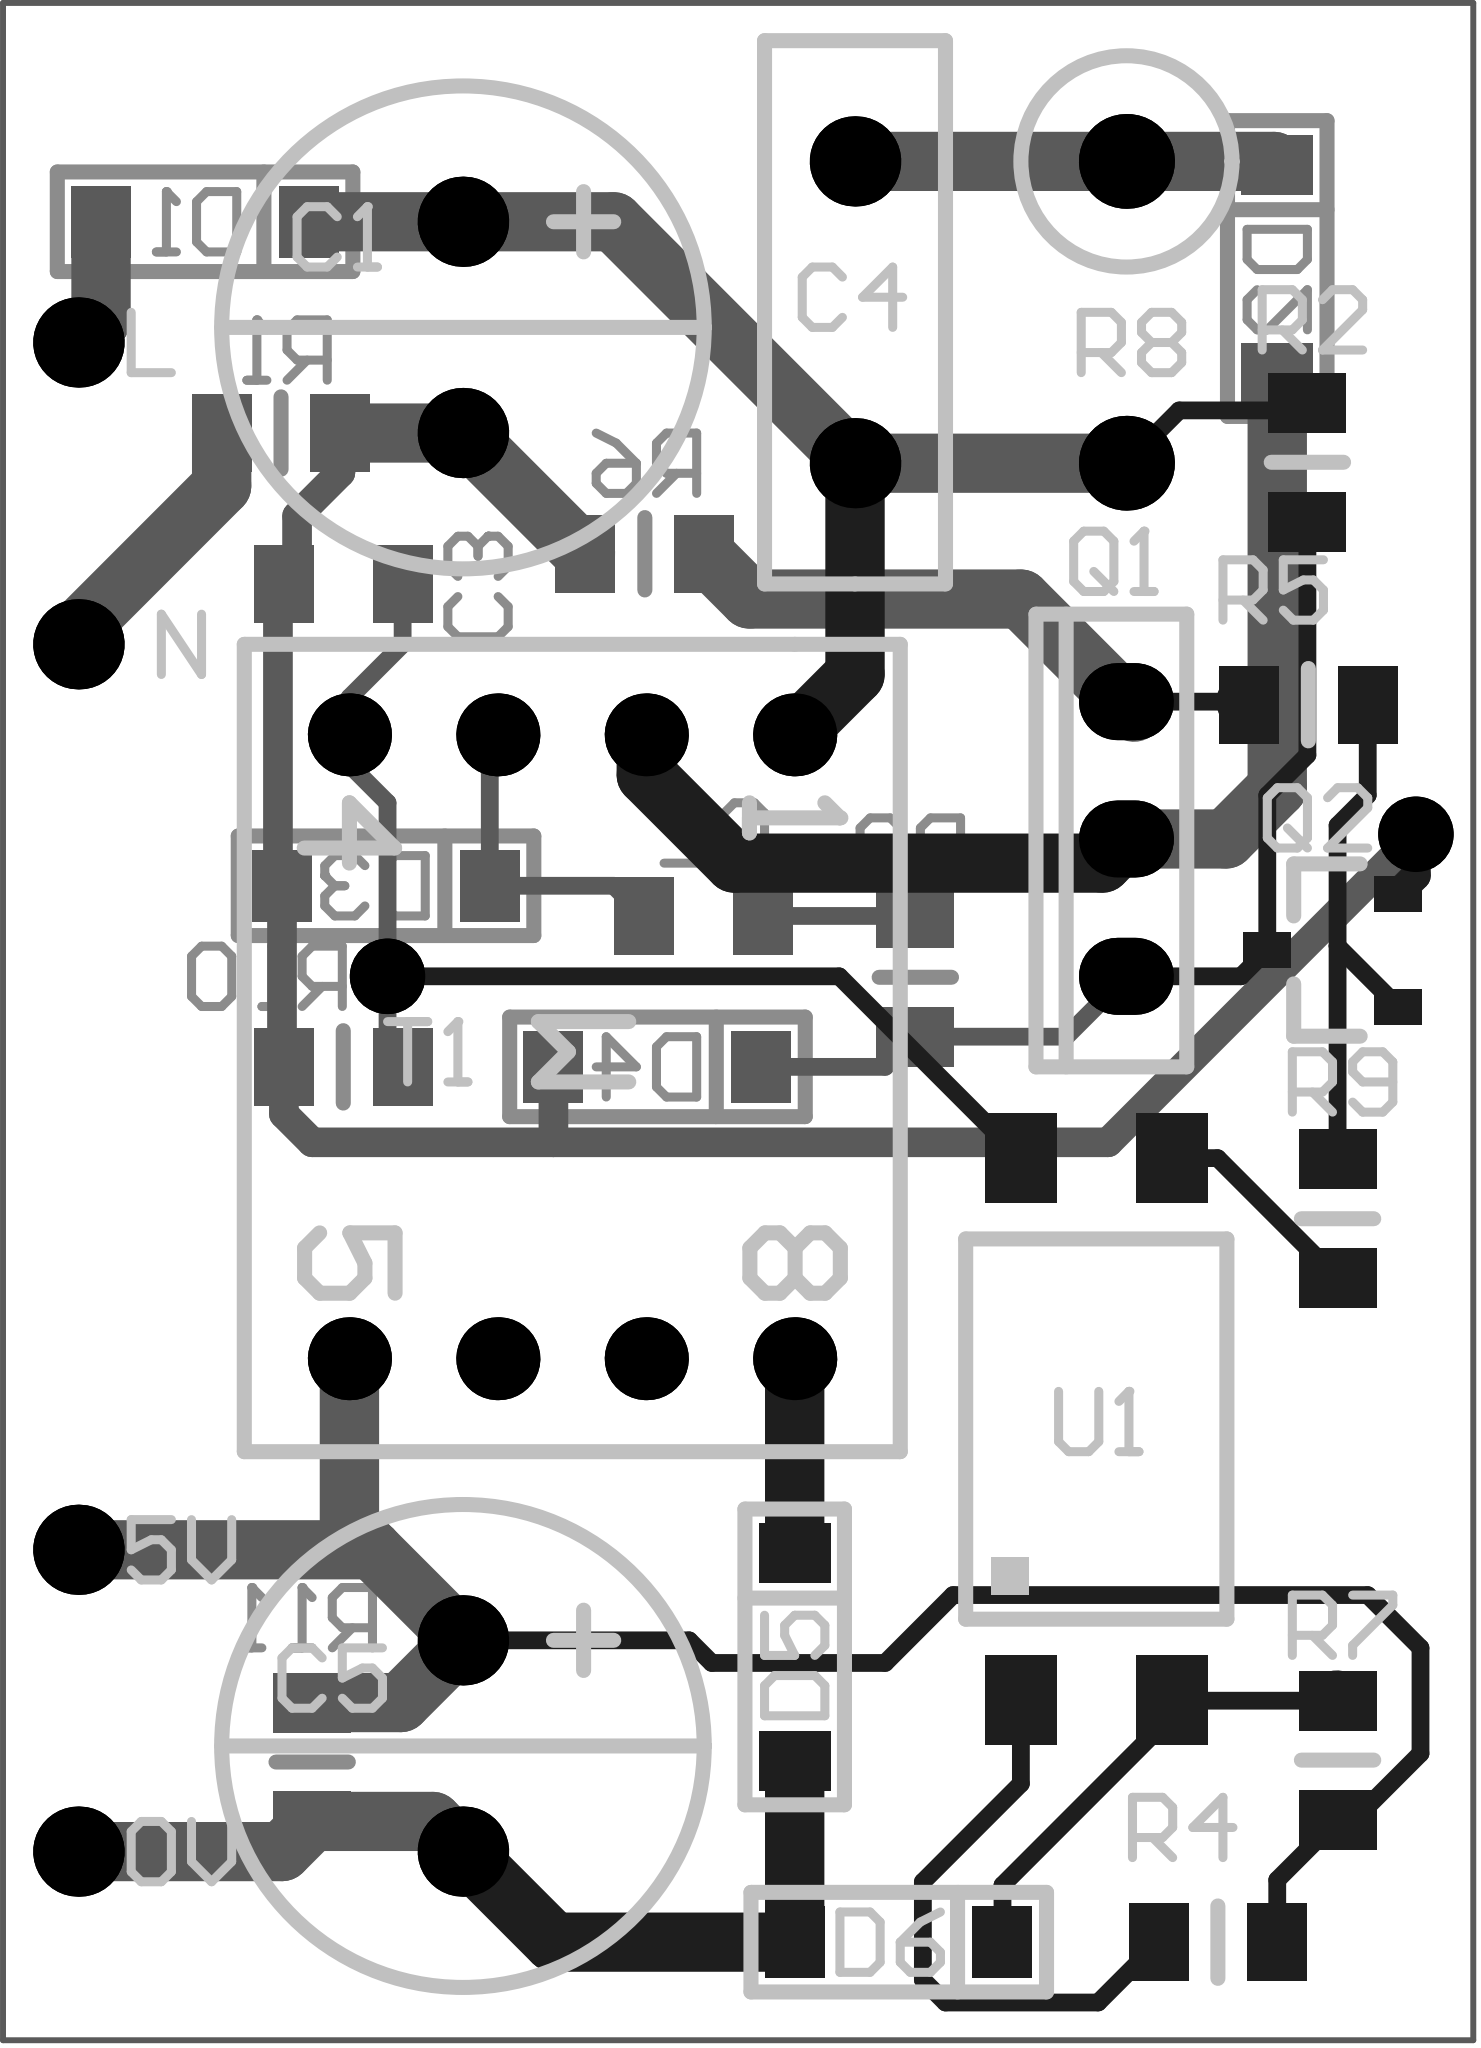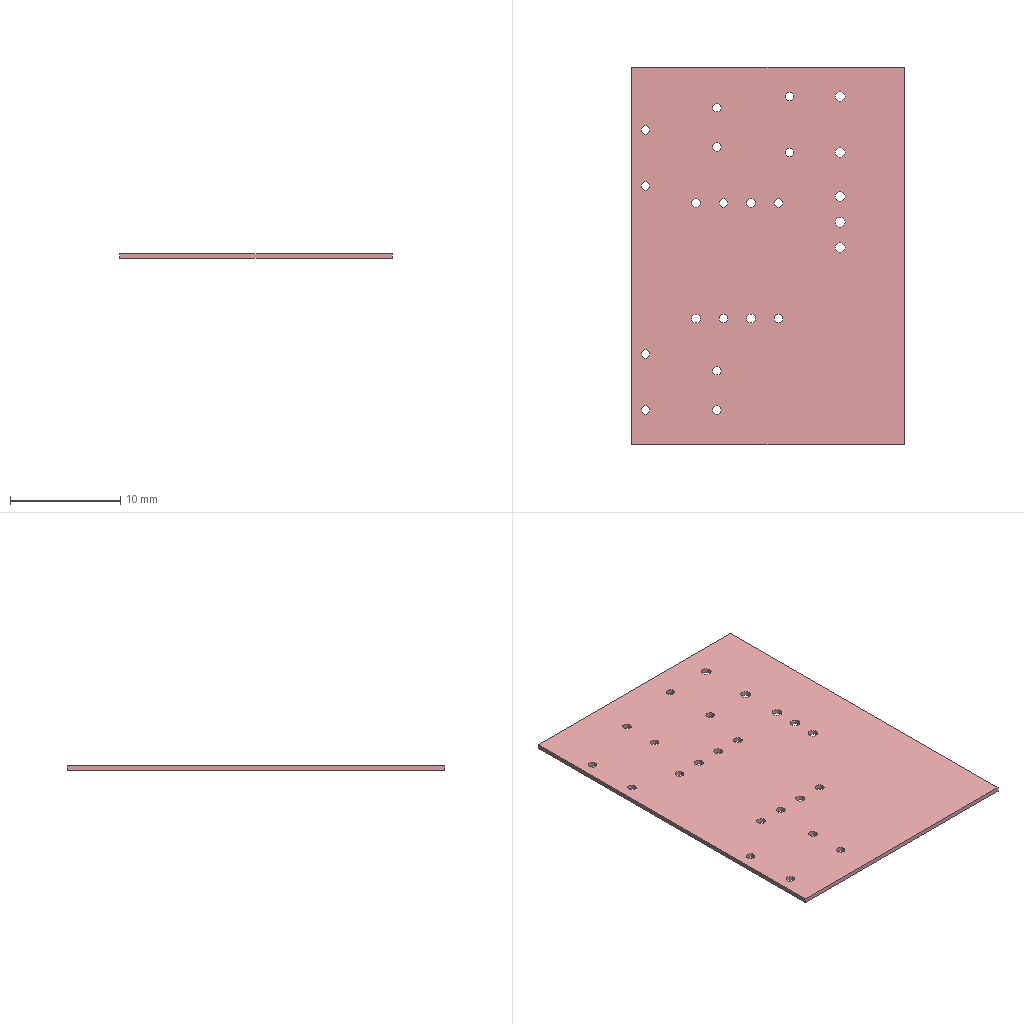Circuit board layout | Altium Designer | box 24.8 x 34.3 x 0.4 mm
Layer stack:
# Altium Designer layer stack of  (unit mm; dielectric type: 0 none, 1 core, 2 prepreg, 3 surface material)
index,name,kind,layer,copper_thickness_mm,dielectric_type,dielectric_thickness_mm,dielectric_material,dielectric_constant
0,Top Paste,other,,,,,,
1,Top Overlay,other,,,,,,
2,Top Solder,dielectric,,,3,0.0102,Solder Resist,3.5
3,Top Layer,copper,Top Layer,0.0356,,,,
4,Dielectric1,dielectric,,,0,0.32,FR-4,4.8
5,Bottom Layer,copper,Bottom Layer,0.0356,,,,
6,Bottom Solder,dielectric,,,3,0.0102,Solder Resist,3.5
7,Bottom Overlay,other,,,,,,
8,Bottom Paste,other,,,,,,
# drill layer pairs: low layer,high layer
drill_pair,Top Layer,Bottom Layer
Part placement:
Designator,Comment,Layer,Footprint,Center-X(mm),Center-Y(mm),Rotation
C1,400V4.7uF,TopLayer,cap-8*14mm,42.672,119.634,270
C2,10nF,BottomLayer,0805_Cap,46.72,109.728,360
C3,16V10uF,BottomLayer,0805_Cap,40.656,115.316,180
C4,1KV4.7nF,TopLayer,CAP_5mm,49.276,119.888,90
C5,16V470uF,TopLayer,cap-8*14mm,42.672,95.758,270
D1,1N4007,BottomLayer,SOD-123,38.326,121.412,360
D2,FR107,BottomLayer,SOD-123,56.388,120.622,90
D3,1N4148,BottomLayer,SOD-123,41.374,110.236,360
D4,18V,BottomLayer,SOD-123,45.946,107.188,360
D5,B5819W,TopLayer,SOD-123,48.26,97.254,90
D6,3.9V,TopLayer,SOD-123,50.01,92.456,360
Q1,1N60,TopLayer,TO-126,53.848,111.023,90
Q2,J3,TopLayer,SOT23,57.32,109.154,90
R1,10R,BottomLayer,0805_Res,39.608,117.856,360
R2,2.2M,TopLayer,0805_Res,56.896,117.364,270
R3,1K,BottomLayer,0805_Res,50.292,108.696,90
R4,10R,TopLayer,0805_Res,55.388,92.456,180
R5,200R,TopLayer,0805_Res,56.912,113.284,180
R6,4.7R,BottomLayer,0805_Res,45.736,115.824,180
R7,200R,TopLayer,0805_Res,57.404,95.52,270
R8,82K/1W,TopLayer,1W_Res_L,53.848,119.888,270
R9,200R,TopLayer,0805_Res,57.404,104.632,90
R10,10K,BottomLayer,0805_Res,40.656,107.188,180
R11,1K,BottomLayer,0805_Res,40.132,95.488,90
T1,EE10_4+4_W,TopLayer,EE10_4+4_W,44.51,107.526,270
U1,PC817,TopLayer,SOP4-PC817,53.34,101.092,90
Pad and via stacks:
# Altium Designer via and pad stacks of  (unit mm). Each distinct definition once, with the count of objects using it.
# via: kind,start_layer,end_layer,hole_mm,diameter_mm,mode(0 simple;1 top-mid-bottom;2 full stack),diameter_per_layer,count,example_net
# pad: kind,layer,hole_mm,hole_type(0 round;1 square;2 slot),plating,top_size,top_shape(1 round;2 rect;3 octagon;9 rounded rect),mid_size,bottom_size,mode,footprint,size_per_layer,count,example
pad,Multi-Layer,0.762,0,plated,1.524x1.524,1,1.524x1.524,1.524x1.524,0,,,4,3
pad,Multi-Layer,0.9,0,plated,1.3x1.6,1,1.3x1.6,1.3x1.6,0,TO-126,,3,Q1.1
pad,Multi-Layer,0.9,0,plated,1.6x1.6,1,1.6x1.6,1.6x1.6,0,1W_Res_L,,2,R8.1
pad,Multi-Layer,0.762,0,plated,1.524x1.524,1,1.524x1.524,1.524x1.524,0,CAP_5mm,,2,C4.1
pad,Multi-Layer,0.8,0,plated,1.4x1.4,1,1.4x1.4,1.4x1.4,0,EE10_4+4_W,,8,T1.5
pad,Multi-Layer,0.762,0,plated,1.524x1.524,1,1.524x1.524,1.524x1.524,0,cap-8*14mm,,4,C1.1
pad,Top Layer,0,0,plated,1x1.3,2,1x1.3,1x1.3,0,0805_Res,,10,R7.2
pad,Top Layer,0,0,plated,1x1.2,2,1x1.2,1x1.2,0,SOD-123,,4,D6.1
pad,Top Layer,0,0,plated,1.5x1.2,2,1.5x1.2,1.5x1.2,0,SOP4-PC817,,4,U1.3
pad,Top Layer,0,0,plated,0.6x0.8,2,0.6x0.8,0.6x0.8,0,SOT23,,3,Q2.3
pad,Bottom Layer,0,0,plated,1x1.3,2,1x1.3,1x1.3,0,0805_Res,,10,R11.2
pad,Bottom Layer,0,0,plated,1x1.2,2,1x1.2,1x1.2,0,SOD-123,,8,D4.1
pad,Bottom Layer,0,0,plated,1x1.3,2,1x1.3,1x1.3,0,0805_Cap,,4,C3.1
via,Top Layer,Bottom Layer,0.7112,1.27,0,,2,HGND
Design rules, without the lines most boards share:
# Altium Designer design rules of  (exported by Altium Designer, unit mm)
# columns: name | kind | enabled | priority | scope1 | scope2 | descriptor | typed fields (field=value)
Clearance | 0 | enabled | 1 | All | All | Clearance Constraint (Gap=0.254mm) (All),(All) | gap=0.254
PlaneConnect | 6 | enabled | 1 | All | All | Power Plane Connect Rule(Relief Connect )(Expansion=0.508mm) (Conductor Width=0.254mm) (Air Gap=0.254mm) (Entries=4) (All) | relief_conductor_width=0.254 relief_entries=4 relief_expansion=0.508
PlaneClearance | 12 | enabled | 1 | All | All | Power Plane Clearance (Clearance =0.508mm) (All) | clearance=0.508
PolygonConnect | 20 | enabled | 1 | All | All | Polygon Connect Rule(Relief Connect )(Conductor Width=0.254mm) (Relief Angle=90 Angle) (Entries=4) (Air Gap Width=0.254mm) (All),(All) | connect_style(0=relief,1=direct,2=none)=0 relief_conductor_width=0.254 relief_entries=4
Width | 2 | enabled | 1 | All | All | Width Constraint (Min=0.3mm) (Max=1.5mm) (Preferred=1mm) (All) |
RoutingCorners | 10 | enabled | 1 | All | All | Routing Corners (Style=45-Degree) (Min Setback=2.54mm) (Max Setback=2.54mm) (All) |
RoutingVias | 11 | enabled | 1 | All | All | Routing Via (MinHoleWidth=0.711mm) (MaxHoleWidth=0.711mm) (PreferredHoleWidth=0.711mm) (MinWidth=1.27mm) (MaxWidth=1.27mm) (PreferedWidth=1.27mm) (All) | via_min_hole=0.7112 via_max_hole=0.7112 via_preferred_diameter=1.27 via_preferred_hole=0.7112
PasteMaskExpansion | 14 | enabled | 1 | All | All | Paste Mask Expansion (Expansion =0mm) (All) | expansion=0
SolderMaskExpansion | 13 | enabled | 1 | All | All | Solder Mask Expansion (Expansion =0.102mm) (All) | expansion=0.1016
ComponentClearance | 24 | enabled | 1 | All | All | Component Clearance Constraint ( Horizontal Gap = 0.254mm, Vertical Gap = 0.254mm ) (All),(All)  | gap=0.254
Height | 50 | enabled | 1 | All | All | Height Constraint (Min=0mm) (Max=25.4mm) (Prefered=12.7mm) (All) | min_height=0 max_height=25.4
HoleSize | 42 | enabled | 1 | All | All | Hole Size Constraint (Min=0.025mm) (Max=2.54mm) (All) |
DiffPairsRouting | 51 | enabled | 1 | All | All | Differential Pairs Uncoupled Length using the Gap Constraints (Min=0.254mm) (Max=0.254mm) (Prefered=0.254mm)  and Width Constraints (Min=0.381mm) (Max=0.381mm) (Prefered=0.381mm) (All) |
HoleToHoleClearance | 52 | enabled | 1 | All | All | Hole To Hole Clearance (Gap=0.254mm) (All),(All) | gap=0.254
MinimumSolderMaskSliver | 53 | enabled | 1 | All | All | Minimum Solder Mask Sliver (Gap=0.254mm) (All),(All) |
SilkscreenOverComponentPads | 54 | enabled | 1 | IsPad | All | Silk To Solder Mask (Clearance=0.254mm) (IsPad),(All) |
SilkToSilkClearance | 55 | enabled | 1 | All | All | Silk to Silk (Clearance=0.254mm) (All),(All) |
NetAntennae | 56 | enabled | 1 | All | All | Net Antennae (Tolerance=0mm) (All) |
Classes set for this board:
# Altium Designer classes of  (member kind: 0 net, 1 component, 2 from-to, 3 pad, 4 layer, 5 differential pair, 6 design channel, 7 polygon, 8 structure, 9 xSignal)
# columns: class name | member kind | superclass | members
5V2W_RCC | 1 | no | C1; C2; C3; C4; C5; D1; D2; D3; D4; D5; D6; Q1; Q2; R1; R2; R3; R4; R5; R6; R7; R8; R9; R10; R11; T1; U1;